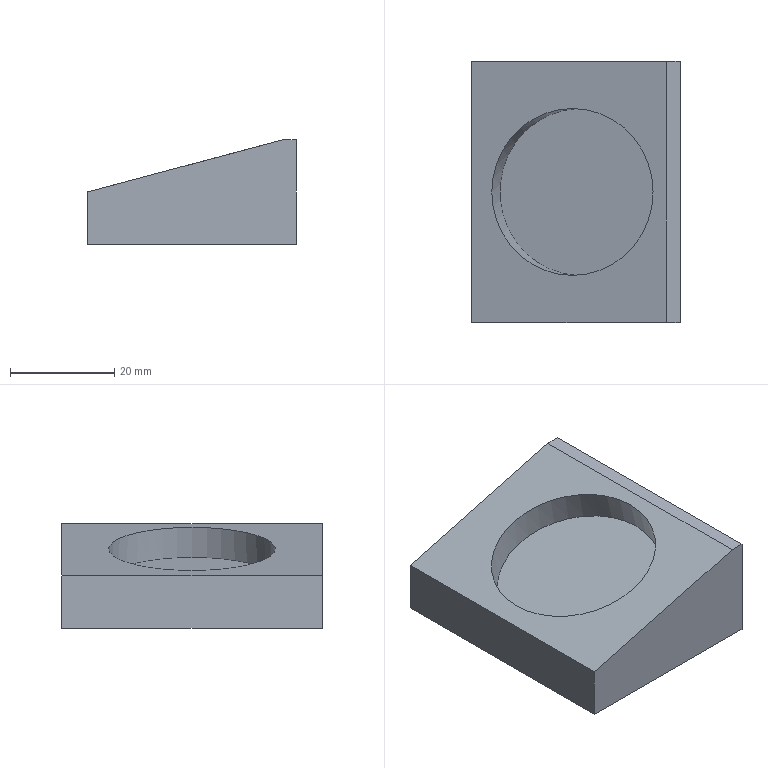Part | NX | features solid 2 | 1 solid | 9 faces | box 40 x 50 x 20 mm | volume 25844 mm3 | plane 8 | cylinder 1 | commonest cylinder face diameters 32 x1
STEP:
#1=CARTESIAN_POINT('',(-677.136,153.,-33.965));
#2=VERTEX_POINT('',#1);
#3=CARTESIAN_POINT('',(-661.681,153.,-29.824));
#4=DIRECTION('',(-0.2588,0.,0.9659));
#5=DIRECTION('',(-0.9659,0.,-0.2588));
#6=AXIS2_PLACEMENT_3D('',#3,#4,#5);
#7=CIRCLE('',#6,16.);
#8=EDGE_CURVE('',#2,#2,#7,.T.);
#9=ORIENTED_EDGE('',*,*,#8,.F.);
#10=EDGE_LOOP('',(#9));
#11=FACE_BOUND('',#10,.T.);
#12=CARTESIAN_POINT('',(-681.,128.,-35.));
#13=VERTEX_POINT('',#12);
#14=CARTESIAN_POINT('',(-643.679,128.,-25.));
#15=VERTEX_POINT('',#14);
#16=CARTESIAN_POINT('',(-683.5,128.,-35.67));
#17=DIRECTION('',(0.9659,0.,0.2588));
#18=VECTOR('',#17,1000.);
#19=LINE('',#16,#18);
#20=EDGE_CURVE('',#13,#15,#19,.T.);
#21=ORIENTED_EDGE('',*,*,#20,.T.);
#22=CARTESIAN_POINT('',(-643.679,178.,-25.));
#23=VERTEX_POINT('',#22);
#24=CARTESIAN_POINT('',(-643.679,178.,-25.));
#25=DIRECTION('',(0.,-1.,0.));
#26=VECTOR('',#25,1000.);
#27=LINE('',#24,#26);
#28=EDGE_CURVE('',#15,#23,#27,.F.);
#29=ORIENTED_EDGE('',*,*,#28,.T.);
#30=CARTESIAN_POINT('',(-681.,178.,-35.));
#31=VERTEX_POINT('',#30);
#32=CARTESIAN_POINT('',(-630.019,178.,-21.34));
#33=DIRECTION('',(-0.9659,0.,-0.2588));
#34=VECTOR('',#33,1000.);
#35=LINE('',#32,#34);
#36=EDGE_CURVE('',#31,#23,#35,.F.);
#37=ORIENTED_EDGE('',*,*,#36,.F.);
#38=CARTESIAN_POINT('',(-681.,178.,-35.));
#39=DIRECTION('',(0.,-1.,0.));
#40=VECTOR('',#39,1000.);
#41=LINE('',#38,#40);
#42=EDGE_CURVE('',#31,#13,#41,.T.);
#43=ORIENTED_EDGE('',*,*,#42,.T.);
#44=EDGE_LOOP('',(#21,#29,#37,#43));
#45=FACE_BOUND('',#44,.T.);
#46=CARTESIAN_POINT('',(-681.,178.,-35.));
#47=DIRECTION('',(-0.2588,0.,0.9659));
#48=DIRECTION('',(-0.9659,0.,-0.2588));
#49=AXIS2_PLACEMENT_3D('',#46,#47,#48);
#50=PLANE('',#49);
#51=ADVANCED_FACE('',(#11,#45),#50,.T.);
#52=CARTESIAN_POINT('',(-641.,128.,-25.));
#53=VERTEX_POINT('',#52);
#54=CARTESIAN_POINT('',(-641.,128.,-25.));
#55=DIRECTION('',(-1.,0.,0.));
#56=VECTOR('',#55,1000.);
#57=LINE('',#54,#56);
#58=EDGE_CURVE('',#15,#53,#57,.F.);
#59=ORIENTED_EDGE('',*,*,#58,.F.);
#60=ORIENTED_EDGE('',*,*,#20,.F.);
#61=CARTESIAN_POINT('',(-681.,128.,-45.));
#62=VERTEX_POINT('',#61);
#63=CARTESIAN_POINT('',(-681.,128.,-45.));
#64=DIRECTION('',(0.,0.,1.));
#65=VECTOR('',#64,1000.);
#66=LINE('',#63,#65);
#67=EDGE_CURVE('',#62,#13,#66,.T.);
#68=ORIENTED_EDGE('',*,*,#67,.F.);
#69=CARTESIAN_POINT('',(-641.,128.,-45.));
#70=VERTEX_POINT('',#69);
#71=CARTESIAN_POINT('',(-681.,128.,-45.));
#72=DIRECTION('',(-1.,0.,0.));
#73=VECTOR('',#72,1000.);
#74=LINE('',#71,#73);
#75=EDGE_CURVE('',#62,#70,#74,.F.);
#76=ORIENTED_EDGE('',*,*,#75,.T.);
#77=CARTESIAN_POINT('',(-641.,128.,-50.));
#78=DIRECTION('',(0.,0.,1.));
#79=VECTOR('',#78,1000.);
#80=LINE('',#77,#79);
#81=EDGE_CURVE('',#70,#53,#80,.T.);
#82=ORIENTED_EDGE('',*,*,#81,.T.);
#83=EDGE_LOOP('',(#59,#60,#68,#76,#82));
#84=FACE_BOUND('',#83,.T.);
#85=CARTESIAN_POINT('',(-681.,128.,-45.));
#86=DIRECTION('',(0.,1.,0.));
#87=DIRECTION('',(0.,0.,-1.));
#88=AXIS2_PLACEMENT_3D('',#85,#86,#87);
#89=PLANE('',#88);
#90=ADVANCED_FACE('',(#84),#89,.F.);
#91=ORIENTED_EDGE('',*,*,#36,.T.);
#92=CARTESIAN_POINT('',(-641.,178.,-25.));
#93=VERTEX_POINT('',#92);
#94=CARTESIAN_POINT('',(-641.,178.,-25.));
#95=DIRECTION('',(-1.,0.,0.));
#96=VECTOR('',#95,1000.);
#97=LINE('',#94,#96);
#98=EDGE_CURVE('',#23,#93,#97,.F.);
#99=ORIENTED_EDGE('',*,*,#98,.T.);
#100=CARTESIAN_POINT('',(-641.,178.,-45.));
#101=VERTEX_POINT('',#100);
#102=CARTESIAN_POINT('',(-641.,178.,-50.));
#103=DIRECTION('',(0.,0.,-1.));
#104=VECTOR('',#103,1000.);
#105=LINE('',#102,#104);
#106=EDGE_CURVE('',#101,#93,#105,.F.);
#107=ORIENTED_EDGE('',*,*,#106,.F.);
#108=CARTESIAN_POINT('',(-681.,178.,-45.));
#109=VERTEX_POINT('',#108);
#110=CARTESIAN_POINT('',(-681.,178.,-45.));
#111=DIRECTION('',(1.,0.,0.));
#112=VECTOR('',#111,1000.);
#113=LINE('',#110,#112);
#114=EDGE_CURVE('',#109,#101,#113,.T.);
#115=ORIENTED_EDGE('',*,*,#114,.F.);
#116=CARTESIAN_POINT('',(-681.,178.,-55.));
#117=DIRECTION('',(0.,0.,-1.));
#118=VECTOR('',#117,1000.);
#119=LINE('',#116,#118);
#120=EDGE_CURVE('',#109,#31,#119,.F.);
#121=ORIENTED_EDGE('',*,*,#120,.T.);
#122=EDGE_LOOP('',(#91,#99,#107,#115,#121));
#123=FACE_BOUND('',#122,.T.);
#124=CARTESIAN_POINT('',(-621.,178.,-55.));
#125=DIRECTION('',(0.,-1.,0.));
#126=DIRECTION('',(-1.,0.,0.));
#127=AXIS2_PLACEMENT_3D('',#124,#125,#126);
#128=PLANE('',#127);
#129=ADVANCED_FACE('',(#123),#128,.F.);
#130=ORIENTED_EDGE('',*,*,#106,.T.);
#131=CARTESIAN_POINT('',(-641.,178.,-25.));
#132=DIRECTION('',(0.,-1.,0.));
#133=VECTOR('',#132,1000.);
#134=LINE('',#131,#133);
#135=EDGE_CURVE('',#93,#53,#134,.T.);
#136=ORIENTED_EDGE('',*,*,#135,.T.);
#137=ORIENTED_EDGE('',*,*,#81,.F.);
#138=CARTESIAN_POINT('',(-641.,178.,-45.));
#139=DIRECTION('',(0.,1.,0.));
#140=VECTOR('',#139,1000.);
#141=LINE('',#138,#140);
#142=EDGE_CURVE('',#101,#70,#141,.F.);
#143=ORIENTED_EDGE('',*,*,#142,.F.);
#144=EDGE_LOOP('',(#130,#136,#137,#143));
#145=FACE_BOUND('',#144,.T.);
#146=CARTESIAN_POINT('',(-641.,158.,-50.));
#147=DIRECTION('',(1.,0.,0.));
#148=DIRECTION('',(0.,-1.,0.));
#149=AXIS2_PLACEMENT_3D('',#146,#147,#148);
#150=PLANE('',#149);
#151=ADVANCED_FACE('',(#145),#150,.T.);
#152=ORIENTED_EDGE('',*,*,#75,.F.);
#153=CARTESIAN_POINT('',(-681.,178.,-45.));
#154=DIRECTION('',(0.,-1.,0.));
#155=VECTOR('',#154,1000.);
#156=LINE('',#153,#155);
#157=EDGE_CURVE('',#62,#109,#156,.F.);
#158=ORIENTED_EDGE('',*,*,#157,.T.);
#159=ORIENTED_EDGE('',*,*,#114,.T.);
#160=ORIENTED_EDGE('',*,*,#142,.T.);
#161=EDGE_LOOP('',(#152,#158,#159,#160));
#162=FACE_BOUND('',#161,.T.);
#163=CARTESIAN_POINT('',(-681.,178.,-45.));
#164=DIRECTION('',(0.,0.,1.));
#165=DIRECTION('',(1.,0.,0.));
#166=AXIS2_PLACEMENT_3D('',#163,#164,#165);
#167=PLANE('',#166);
#168=ADVANCED_FACE('',(#162),#167,.F.);
#169=ORIENTED_EDGE('',*,*,#157,.F.);
#170=ORIENTED_EDGE('',*,*,#67,.T.);
#171=ORIENTED_EDGE('',*,*,#42,.F.);
#172=ORIENTED_EDGE('',*,*,#120,.F.);
#173=EDGE_LOOP('',(#169,#170,#171,#172));
#174=FACE_BOUND('',#173,.T.);
#175=CARTESIAN_POINT('',(-681.,153.5,-40.721));
#176=DIRECTION('',(-1.,0.,0.));
#177=DIRECTION('',(0.,-1.,0.));
#178=AXIS2_PLACEMENT_3D('',#175,#176,#177);
#179=PLANE('',#178);
#180=ADVANCED_FACE('',(#174),#179,.T.);
#181=CARTESIAN_POINT('',(-644.674,153.,-31.478));
#182=VERTEX_POINT('',#181);
#183=CARTESIAN_POINT('',(-660.129,153.,-35.619));
#184=DIRECTION('',(0.2588,0.,-0.9659));
#185=DIRECTION('',(0.9659,0.,0.2588));
#186=AXIS2_PLACEMENT_3D('',#183,#184,#185);
#187=CIRCLE('',#186,16.);
#188=EDGE_CURVE('',#182,#182,#187,.F.);
#189=ORIENTED_EDGE('',*,*,#188,.T.);
#190=EDGE_LOOP('',(#189));
#191=FACE_BOUND('',#190,.T.);
#192=CARTESIAN_POINT('',(-659.836,153.,-35.541));
#193=DIRECTION('',(0.2588,0.,-0.9659));
#194=DIRECTION('',(0.01205,-0.9999,0.003228));
#195=AXIS2_PLACEMENT_3D('',#192,#193,#194);
#196=PLANE('',#195);
#197=ADVANCED_FACE('',(#191),#196,.F.);
#198=ORIENTED_EDGE('',*,*,#8,.T.);
#199=EDGE_LOOP('',(#198));
#200=FACE_BOUND('',#199,.T.);
#201=ORIENTED_EDGE('',*,*,#188,.F.);
#202=EDGE_LOOP('',(#201));
#203=FACE_BOUND('',#202,.T.);
#204=CARTESIAN_POINT('',(-661.681,153.,-29.824));
#205=DIRECTION('',(0.2588,0.,-0.9659));
#206=DIRECTION('',(0.01205,-0.9999,0.003228));
#207=AXIS2_PLACEMENT_3D('',#204,#205,#206);
#208=CYLINDRICAL_SURFACE('',#207,16.);
#209=ADVANCED_FACE('',(#200,#203),#208,.F.);
#210=ORIENTED_EDGE('',*,*,#58,.T.);
#211=ORIENTED_EDGE('',*,*,#135,.F.);
#212=ORIENTED_EDGE('',*,*,#98,.F.);
#213=ORIENTED_EDGE('',*,*,#28,.F.);
#214=EDGE_LOOP('',(#210,#211,#212,#213));
#215=FACE_BOUND('',#214,.T.);
#216=CARTESIAN_POINT('',(-641.,178.,-25.));
#217=DIRECTION('',(0.,0.,-1.));
#218=DIRECTION('',(0.,-1.,0.));
#219=AXIS2_PLACEMENT_3D('',#216,#217,#218);
#220=PLANE('',#219);
#221=ADVANCED_FACE('',(#215),#220,.F.);
#222=CLOSED_SHELL('',(#51,#90,#129,#151,#168,#180,#197,#209,#221));
#223=MANIFOLD_SOLID_BREP('',#222);
#224=(LENGTH_UNIT()NAMED_UNIT(*)SI_UNIT(.MILLI.,.METRE.));
#225=UNCERTAINTY_MEASURE_WITH_UNIT(LENGTH_MEASURE(0.00001),#224,'','');
#226=(NAMED_UNIT(*)PLANE_ANGLE_UNIT()SI_UNIT($,.RADIAN.));
#227=(NAMED_UNIT(*)SI_UNIT($,.STERADIAN.)SOLID_ANGLE_UNIT());
#228=(GEOMETRIC_REPRESENTATION_CONTEXT(3)GLOBAL_UNCERTAINTY_ASSIGNED_CONTEXT((#225))GLOBAL_UNIT_ASSIGNED_CONTEXT((#224,#226,#227))REPRESENTATION_CONTEXT('',''));
#229=ADVANCED_BREP_SHAPE_REPRESENTATION('',(#223),#228);